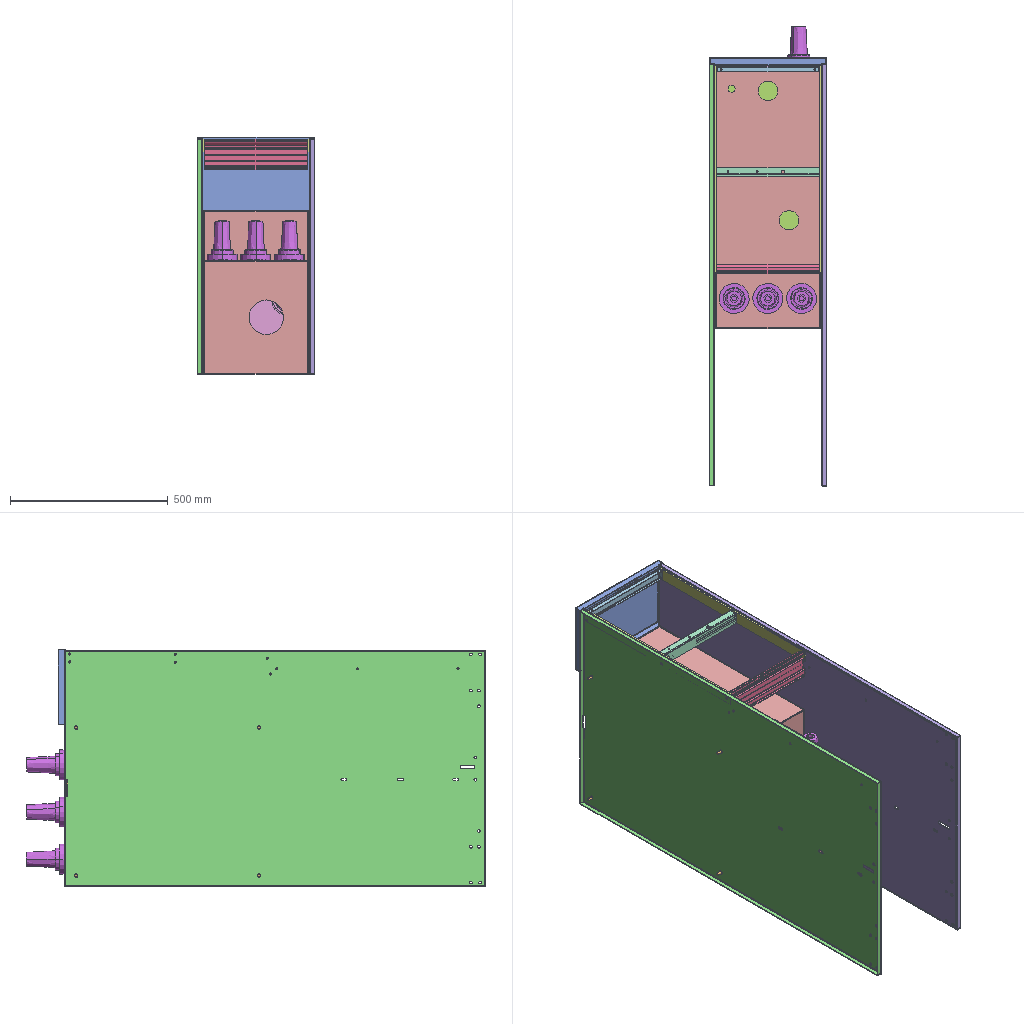Assembly | SolidWorks | 13 different items | 19 placed | box 371 x 1460 x 753 mm
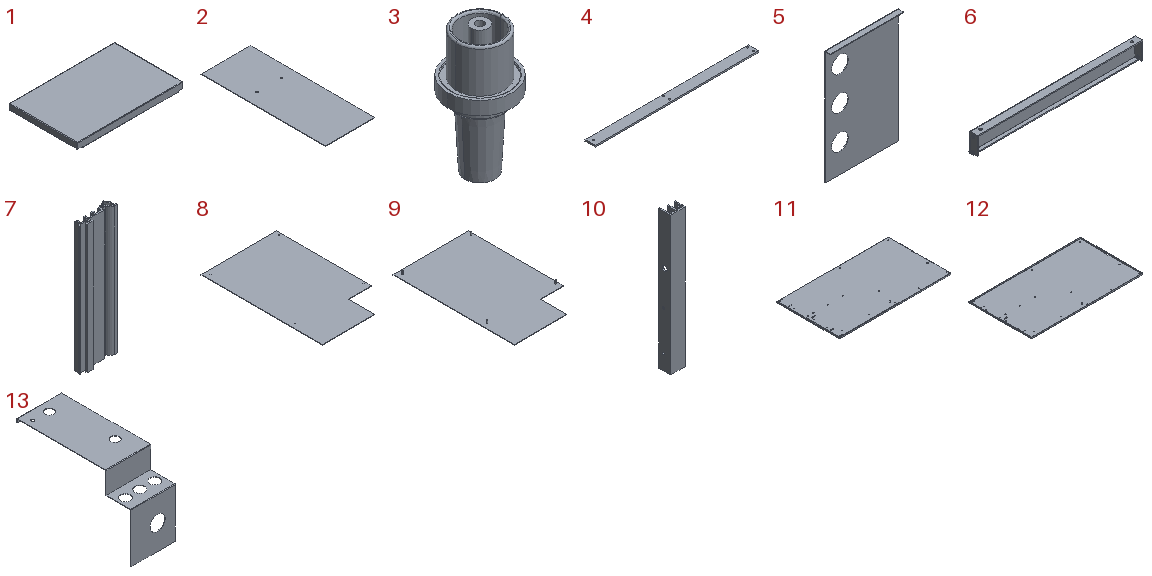Parts list (item | quantity | size | volume | features):
1 | x1 | 371 x 240 x 23.8 mm | 183255 mm3 | features EdgeFlange 7, FlatPattern 1, ICE 1, SMBaseFlange 1, SheetMetal 1
2 | x1 | 325 x 820 x 3 mm | 798821 mm3 | features Extrusion 1, ICE 1
3 | x6 | 96 x 96 x 193 mm | 497884 mm3 | features ICE 9, Fillet 4, Extrusion 1
4 | x2 | 655 x 40 x 6 mm | 156045 mm3 | features FlatPattern 1, SMBaseFlange 1, SheetMetal 1
5 | x1 | 325 x 25 x 508 mm | 477331 mm3 | features EdgeFlange 1, FlatPattern 1, ICE 1, SMBaseFlange 1, SheetMetal 1
6 | x1 | 325 x 16 x 37 mm | 38534 mm3 | features EdgeFlange 4, ICE 2, FlatPattern 1, SMBaseFlange 1, SheetMetal 1
7 | x1 | 96.9 x 30 x 325 mm | 198402 mm3 | features Extrusion 1
8 | x1 | 520 x 833 x 23 mm | 1217641 mm3 | features FlatPattern 1, ICE 1, SMBaseFlange 1, SheetMetal 1
9 | x1 | 520 x 833 x 23 mm | 1217641 mm3 | features ICE 2, FlatPattern 1, SMBaseFlange 1, SheetMetal 1
10 | x1 | 35 x 28 x 325 mm | 111958 mm3 | features ICE 2, Extrusion 1
11 | x1 | 1338 x 750 x 17 mm | 3164548 mm3 | features EdgeFlange 4, FlatPattern 1, ICE 1, SMBaseFlange 1, SheetMetal 1
12 | x1 | 1338 x 750 x 17 mm | 3164548 mm3 | features EdgeFlange 4, FlatPattern 1, ICE 1, SMBaseFlange 1, SheetMetal 1
13 | x1 | 325 x 830 x 520 mm | 1245457 mm3 | features EdgeFlange 4, ICE 4, FlatPattern 1, SMBaseFlange 1, SheetMetal 1
Mates (type | each side: item.copy, entity, surface, feature):
Coincident | 13.1 face plane Base-Flange1 | 9.1 face plane Base-Flange1 | 2 times
Coincident | 13.1 face plane Edge-Flange5 | 9.1 face plane Base-Flange1
Coincident | 13.1 face plane Edge-Flange4 | 8.1 face plane Base-Flange1
Coincident | 13.1 face plane Base-Flange1 | 8.1 face plane Base-Flange1
Coincident | 13.1 face plane Edge-Flange5 | 8.1 face plane Base-Flange1
Coincident | 2.1 face plane Boss-Extrude1 | 8.1 face plane Base-Flange1 | 2 times
Coincident | 13.1 face plane Edge-Flange1 | 5.1 face plane Edge-Flange1
Coincident | 2.1 face plane Boss-Extrude1 | 5.1 face plane Base-Flange1 | 2 times
Coincident | 5.1 face plane Edge-Flange1 | 9.1 face plane Base-Flange1
Coincident | 13.1 face plane Edge-Flange5 | 2.1 face plane Boss-Extrude1
DistanceDim | 9.1 face plane Base-Flange1 | 12.1 face plane Base-Flange1
DistanceDim | 8.1 face plane Base-Flange1 | 11.1 face plane Base-Flange1
Coincident | 11.1 face plane Base-Flange1 | 4.1 face plane Base-Flange1
Concentric | 11.1 face cylinder Base-Flange1 | 4.1 face cylinder Base-Flange1 | 2 times
Coincident | 12.1 face plane Base-Flange1 | 4.2 face plane Base-Flange1
Concentric | 12.1 face cylinder Base-Flange1 | 4.2 face cylinder Base-Flange1 | 2 times
Concentric | 6.1 face cylinder Cut-Extrude1 | 4.1 face cylinder Base-Flange1 | 2 times
Coincident | 6.1 face plane Edge-Flange6 | 4.1 face plane Base-Flange1
Concentric | 7.1 face cylinder Boss-Extrude1 | 4.2 face cylinder Base-Flange1
Concentric | 12.1 face cylinder Base-Flange1 | 7.1 face cylinder Boss-Extrude1
Coincident | 7.1 face plane Boss-Extrude1 | 4.2 face plane Base-Flange1
Coincident | 5.1 face plane Edge-Flange1 | 3.1 face plane Boss-Extrude3
Concentric | 5.1 face cylinder Cut-Extrude3 | 3.1 face cylinder Boss-Extrude1
Coincident | 5.1 face plane Edge-Flange1 | 3.2 face plane Boss-Extrude3
Concentric | 5.1 face cylinder Cut-Extrude3 | 3.2 face cylinder Boss-Extrude1
Coincident | 5.1 face plane Edge-Flange1 | 3.3 face plane Boss-Extrude3
Concentric | 5.1 face cylinder Cut-Extrude3 | 3.3 face cylinder Boss-Extrude1
Coincident | 13.1 face plane Edge-Flange4 | 3.4 face plane Boss-Extrude3
Concentric | 13.1 face cylinder Cut-Extrude2 | 3.4 face cylinder Boss-Extrude1
Coincident | 13.1 face plane Edge-Flange4 | 3.5 face plane Boss-Extrude3
Concentric | 13.1 face cylinder Cut-Extrude2 | 3.5 face cylinder Boss-Extrude1
Coincident | 13.1 face plane Edge-Flange4 | 3.6 face plane Boss-Extrude3
Concentric | 13.1 face cylinder Cut-Extrude2 | 3.6 face cylinder Boss-Extrude1
Concentric | 4.1 face cylinder Base-Flange1 | 10.1 face cylinder Boss-Extrude1 | 2 times
Coincident | 4.1 face plane Base-Flange1 | 10.1 face plane Boss-Extrude1
Concentric | 8.1 face cylinder Boss-Extrude1 | 11.1 face cylinder Base-Flange1 | 2 times
Concentric | 9.1 face cylinder Boss-Extrude1 | 12.1 face cylinder Base-Flange1
Coincident | 1.1 face plane Edge-Flange21 | 11.1 face plane Edge-Flange4
Coincident | 1.1 face plane Edge-Flange20 | 11.1 face plane Edge-Flange4